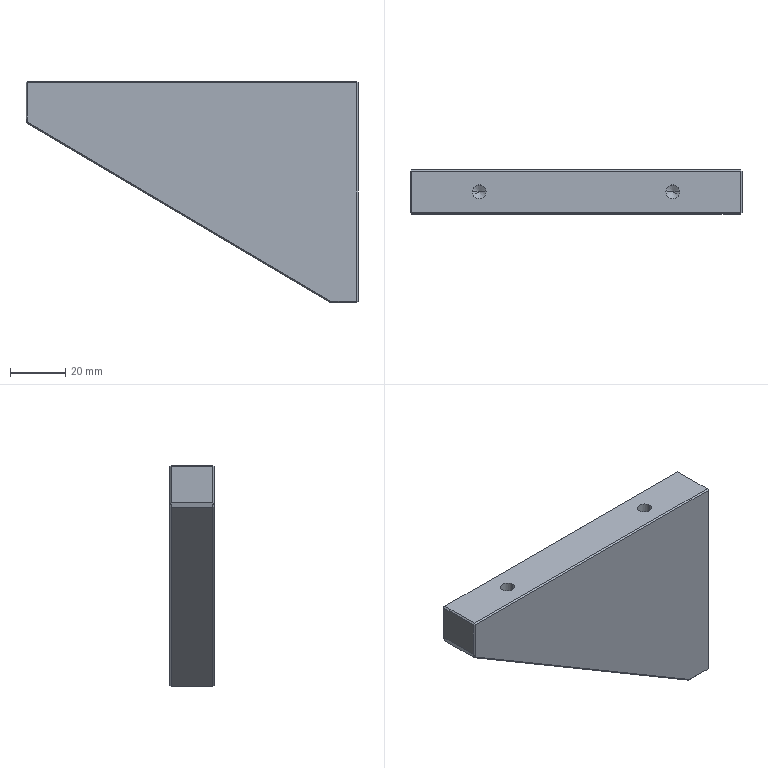Part | STEP file | ND25021-01-JDKM-05-TL | 1 solid | 45 faces | box 120 x 16 x 80 mm | volume 95084 mm3 | plane 29 | cylinder 8 | cone 8 | commonest cylinder face diameters 5 x8